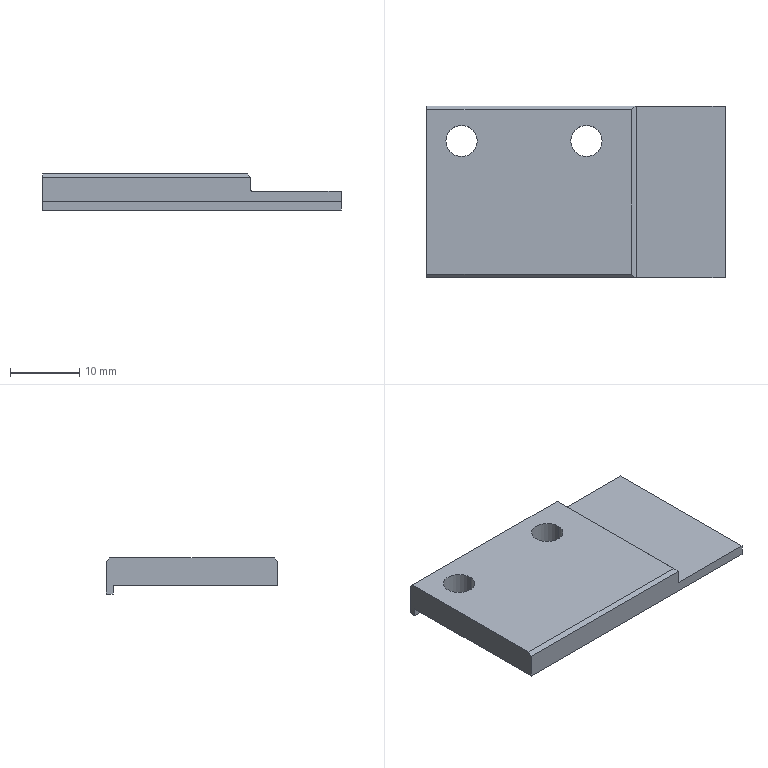Part | NX | 1 solid | 18 faces | box 43 x 24.7 x 5.2 mm | volume 3360 mm3 | plane 13 | cylinder 5 | commonest cylinder face diameters 4.5 x4 0.4 x1
STEP:
#1=CARTESIAN_POINT('',(0.,0.,-0.2));
#2=VERTEX_POINT('',#1);
#3=CARTESIAN_POINT('',(0.,-1.,-0.2));
#4=VERTEX_POINT('',#3);
#5=CARTESIAN_POINT('',(0.,0.,-0.2));
#6=DIRECTION('',(0.,-1.,0.));
#7=VECTOR('',#6,1000.);
#8=LINE('',#5,#7);
#9=EDGE_CURVE('',#2,#4,#8,.T.);
#10=ORIENTED_EDGE('',*,*,#9,.F.);
#11=CARTESIAN_POINT('',(43.,0.,-0.2));
#12=VERTEX_POINT('',#11);
#13=CARTESIAN_POINT('',(0.,0.,-0.2));
#14=DIRECTION('',(1.,0.,0.));
#15=VECTOR('',#14,1000.);
#16=LINE('',#13,#15);
#17=EDGE_CURVE('',#2,#12,#16,.T.);
#18=ORIENTED_EDGE('',*,*,#17,.T.);
#19=CARTESIAN_POINT('',(43.,-1.,-0.2));
#20=VERTEX_POINT('',#19);
#21=CARTESIAN_POINT('',(43.,0.,-0.2));
#22=DIRECTION('',(0.,-1.,0.));
#23=VECTOR('',#22,1000.);
#24=LINE('',#21,#23);
#25=EDGE_CURVE('',#12,#20,#24,.T.);
#26=ORIENTED_EDGE('',*,*,#25,.T.);
#27=CARTESIAN_POINT('',(0.,-1.,-0.2));
#28=DIRECTION('',(-1.,0.,0.));
#29=VECTOR('',#28,1000.);
#30=LINE('',#27,#29);
#31=EDGE_CURVE('',#20,#4,#30,.T.);
#32=ORIENTED_EDGE('',*,*,#31,.T.);
#33=EDGE_LOOP('',(#10,#18,#26,#32));
#34=FACE_BOUND('',#33,.T.);
#35=CARTESIAN_POINT('',(0.,0.,-0.2));
#36=DIRECTION('',(0.,0.,1.));
#37=DIRECTION('',(1.,0.,0.));
#38=AXIS2_PLACEMENT_3D('',#35,#36,#37);
#39=PLANE('',#38);
#40=ADVANCED_FACE('',(#34),#39,.F.);
#41=ORIENTED_EDGE('',*,*,#9,.T.);
#42=CARTESIAN_POINT('',(0.,-1.,1.));
#43=VERTEX_POINT('',#42);
#44=CARTESIAN_POINT('',(0.,-1.,0.));
#45=DIRECTION('',(0.,0.,-1.));
#46=VECTOR('',#45,1000.);
#47=LINE('',#44,#46);
#48=EDGE_CURVE('',#43,#4,#47,.T.);
#49=ORIENTED_EDGE('',*,*,#48,.F.);
#50=CARTESIAN_POINT('',(0.,-24.7,1.));
#51=VERTEX_POINT('',#50);
#52=CARTESIAN_POINT('',(0.,0.,1.));
#53=DIRECTION('',(0.,-1.,0.));
#54=VECTOR('',#53,1000.);
#55=LINE('',#52,#54);
#56=EDGE_CURVE('',#43,#51,#55,.T.);
#57=ORIENTED_EDGE('',*,*,#56,.T.);
#58=CARTESIAN_POINT('',(0.,-24.7,4.5));
#59=VERTEX_POINT('',#58);
#60=CARTESIAN_POINT('',(0.,-24.7,0.));
#61=DIRECTION('',(0.,0.,-1.));
#62=VECTOR('',#61,1000.);
#63=LINE('',#60,#62);
#64=EDGE_CURVE('',#59,#51,#63,.T.);
#65=ORIENTED_EDGE('',*,*,#64,.F.);
#66=CARTESIAN_POINT('',(0.,-24.2,5.));
#67=VERTEX_POINT('',#66);
#68=CARTESIAN_POINT('',(0.,-29.2,0.));
#69=DIRECTION('',(0.,0.7071,0.7071));
#70=VECTOR('',#69,1000.);
#71=LINE('',#68,#70);
#72=EDGE_CURVE('',#59,#67,#71,.T.);
#73=ORIENTED_EDGE('',*,*,#72,.T.);
#74=CARTESIAN_POINT('',(0.,-0.5,5.));
#75=VERTEX_POINT('',#74);
#76=CARTESIAN_POINT('',(0.,0.,5.));
#77=DIRECTION('',(0.,-1.,0.));
#78=VECTOR('',#77,1000.);
#79=LINE('',#76,#78);
#80=EDGE_CURVE('',#75,#67,#79,.T.);
#81=ORIENTED_EDGE('',*,*,#80,.F.);
#82=CARTESIAN_POINT('',(0.,0.,4.5));
#83=VERTEX_POINT('',#82);
#84=CARTESIAN_POINT('',(0.,4.5,0.));
#85=DIRECTION('',(0.,-0.7071,0.7071));
#86=VECTOR('',#85,1000.);
#87=LINE('',#84,#86);
#88=EDGE_CURVE('',#83,#75,#87,.T.);
#89=ORIENTED_EDGE('',*,*,#88,.F.);
#90=CARTESIAN_POINT('',(0.,0.,0.));
#91=DIRECTION('',(0.,0.,1.));
#92=VECTOR('',#91,1000.);
#93=LINE('',#90,#92);
#94=EDGE_CURVE('',#2,#83,#93,.T.);
#95=ORIENTED_EDGE('',*,*,#94,.F.);
#96=EDGE_LOOP('',(#41,#49,#57,#65,#73,#81,#89,#95));
#97=FACE_BOUND('',#96,.T.);
#98=CARTESIAN_POINT('',(0.,0.,0.));
#99=DIRECTION('',(-1.,0.,0.));
#100=DIRECTION('',(0.,0.,1.));
#101=AXIS2_PLACEMENT_3D('',#98,#99,#100);
#102=PLANE('',#101);
#103=ADVANCED_FACE('',(#97),#102,.T.);
#104=CARTESIAN_POINT('',(30.,0.,4.5));
#105=VERTEX_POINT('',#104);
#106=CARTESIAN_POINT('',(0.,0.,4.5));
#107=DIRECTION('',(-1.,0.,0.));
#108=VECTOR('',#107,1000.);
#109=LINE('',#106,#108);
#110=EDGE_CURVE('',#105,#83,#109,.T.);
#111=ORIENTED_EDGE('',*,*,#110,.F.);
#112=CARTESIAN_POINT('',(30.,0.,2.7));
#113=VERTEX_POINT('',#112);
#114=CARTESIAN_POINT('',(30.,0.,0.));
#115=DIRECTION('',(0.,0.,-1.));
#116=VECTOR('',#115,1000.);
#117=LINE('',#114,#116);
#118=EDGE_CURVE('',#105,#113,#117,.T.);
#119=ORIENTED_EDGE('',*,*,#118,.T.);
#120=CARTESIAN_POINT('',(30.2,0.,2.5));
#121=VERTEX_POINT('',#120);
#122=CARTESIAN_POINT('',(30.2,0.,2.7));
#123=DIRECTION('',(0.,1.,0.));
#124=DIRECTION('',(0.,0.,-1.));
#125=AXIS2_PLACEMENT_3D('',#122,#123,#124);
#126=CIRCLE('',#125,0.2);
#127=EDGE_CURVE('',#121,#113,#126,.T.);
#128=ORIENTED_EDGE('',*,*,#127,.F.);
#129=CARTESIAN_POINT('',(43.,0.,2.5));
#130=VERTEX_POINT('',#129);
#131=CARTESIAN_POINT('',(0.,0.,2.5));
#132=DIRECTION('',(-1.,0.,0.));
#133=VECTOR('',#132,1000.);
#134=LINE('',#131,#133);
#135=EDGE_CURVE('',#130,#121,#134,.T.);
#136=ORIENTED_EDGE('',*,*,#135,.F.);
#137=CARTESIAN_POINT('',(43.,0.,0.));
#138=DIRECTION('',(0.,0.,1.));
#139=VECTOR('',#138,1000.);
#140=LINE('',#137,#139);
#141=EDGE_CURVE('',#12,#130,#140,.T.);
#142=ORIENTED_EDGE('',*,*,#141,.F.);
#143=ORIENTED_EDGE('',*,*,#17,.F.);
#144=ORIENTED_EDGE('',*,*,#94,.T.);
#145=EDGE_LOOP('',(#111,#119,#128,#136,#142,#143,#144));
#146=FACE_BOUND('',#145,.T.);
#147=CARTESIAN_POINT('',(43.,0.,0.));
#148=DIRECTION('',(0.,1.,0.));
#149=DIRECTION('',(1.,0.,0.));
#150=AXIS2_PLACEMENT_3D('',#147,#148,#149);
#151=PLANE('',#150);
#152=ADVANCED_FACE('',(#146),#151,.T.);
#153=CARTESIAN_POINT('',(30.2,-24.7,2.5));
#154=VERTEX_POINT('',#153);
#155=CARTESIAN_POINT('',(30.2,-26.782,2.5));
#156=DIRECTION('',(0.,1.,0.));
#157=VECTOR('',#156,1000.);
#158=LINE('',#155,#157);
#159=EDGE_CURVE('',#154,#121,#158,.T.);
#160=ORIENTED_EDGE('',*,*,#159,.F.);
#161=CARTESIAN_POINT('',(43.,-24.7,2.5));
#162=VERTEX_POINT('',#161);
#163=CARTESIAN_POINT('',(0.,-24.7,2.5));
#164=DIRECTION('',(-1.,0.,0.));
#165=VECTOR('',#164,1000.);
#166=LINE('',#163,#165);
#167=EDGE_CURVE('',#162,#154,#166,.T.);
#168=ORIENTED_EDGE('',*,*,#167,.F.);
#169=CARTESIAN_POINT('',(43.,0.,2.5));
#170=DIRECTION('',(0.,1.,0.));
#171=VECTOR('',#170,1000.);
#172=LINE('',#169,#171);
#173=EDGE_CURVE('',#162,#130,#172,.T.);
#174=ORIENTED_EDGE('',*,*,#173,.T.);
#175=ORIENTED_EDGE('',*,*,#135,.T.);
#176=EDGE_LOOP('',(#160,#168,#174,#175));
#177=FACE_BOUND('',#176,.T.);
#178=CARTESIAN_POINT('',(0.,0.,2.5));
#179=DIRECTION('',(0.,0.,1.));
#180=DIRECTION('',(1.,0.,0.));
#181=AXIS2_PLACEMENT_3D('',#178,#179,#180);
#182=PLANE('',#181);
#183=ADVANCED_FACE('',(#177),#182,.T.);
#184=ORIENTED_EDGE('',*,*,#159,.T.);
#185=ORIENTED_EDGE('',*,*,#127,.T.);
#186=CARTESIAN_POINT('',(30.,-24.7,2.7));
#187=VERTEX_POINT('',#186);
#188=CARTESIAN_POINT('',(30.,-26.7,2.7));
#189=DIRECTION('',(0.,1.,0.));
#190=VECTOR('',#189,1000.);
#191=LINE('',#188,#190);
#192=EDGE_CURVE('',#187,#113,#191,.T.);
#193=ORIENTED_EDGE('',*,*,#192,.F.);
#194=CARTESIAN_POINT('',(30.2,-24.7,2.7));
#195=DIRECTION('',(0.,1.,0.));
#196=DIRECTION('',(0.,0.,-1.));
#197=AXIS2_PLACEMENT_3D('',#194,#195,#196);
#198=CIRCLE('',#197,0.2);
#199=EDGE_CURVE('',#154,#187,#198,.T.);
#200=ORIENTED_EDGE('',*,*,#199,.F.);
#201=EDGE_LOOP('',(#184,#185,#193,#200));
#202=FACE_BOUND('',#201,.T.);
#203=CARTESIAN_POINT('',(30.2,-26.782,2.7));
#204=DIRECTION('',(0.,1.,0.));
#205=DIRECTION('',(0.,0.,-1.));
#206=AXIS2_PLACEMENT_3D('',#203,#204,#205);
#207=CYLINDRICAL_SURFACE('',#206,0.2);
#208=ADVANCED_FACE('',(#202),#207,.F.);
#209=CARTESIAN_POINT('',(30.,-24.7,4.5));
#210=VERTEX_POINT('',#209);
#211=CARTESIAN_POINT('',(0.,-24.7,4.5));
#212=DIRECTION('',(-1.,0.,0.));
#213=VECTOR('',#212,1000.);
#214=LINE('',#211,#213);
#215=EDGE_CURVE('',#210,#59,#214,.T.);
#216=ORIENTED_EDGE('',*,*,#215,.T.);
#217=ORIENTED_EDGE('',*,*,#64,.T.);
#218=CARTESIAN_POINT('',(43.,-24.7,1.));
#219=VERTEX_POINT('',#218);
#220=CARTESIAN_POINT('',(0.,-24.7,1.));
#221=DIRECTION('',(-1.,0.,0.));
#222=VECTOR('',#221,1000.);
#223=LINE('',#220,#222);
#224=EDGE_CURVE('',#219,#51,#223,.T.);
#225=ORIENTED_EDGE('',*,*,#224,.F.);
#226=CARTESIAN_POINT('',(43.,-24.7,0.));
#227=DIRECTION('',(0.,0.,1.));
#228=VECTOR('',#227,1000.);
#229=LINE('',#226,#228);
#230=EDGE_CURVE('',#219,#162,#229,.T.);
#231=ORIENTED_EDGE('',*,*,#230,.T.);
#232=ORIENTED_EDGE('',*,*,#167,.T.);
#233=ORIENTED_EDGE('',*,*,#199,.T.);
#234=CARTESIAN_POINT('',(30.,-24.7,0.));
#235=DIRECTION('',(0.,0.,1.));
#236=VECTOR('',#235,1000.);
#237=LINE('',#234,#236);
#238=EDGE_CURVE('',#187,#210,#237,.T.);
#239=ORIENTED_EDGE('',*,*,#238,.T.);
#240=EDGE_LOOP('',(#216,#217,#225,#231,#232,#233,#239));
#241=FACE_BOUND('',#240,.T.);
#242=CARTESIAN_POINT('',(0.,-24.7,0.));
#243=DIRECTION('',(0.,-1.,0.));
#244=DIRECTION('',(0.,0.,-1.));
#245=AXIS2_PLACEMENT_3D('',#242,#243,#244);
#246=PLANE('',#245);
#247=ADVANCED_FACE('',(#241),#246,.T.);
#248=CARTESIAN_POINT('',(30.,0.,4.5));
#249=DIRECTION('',(0.,1.,0.));
#250=VECTOR('',#249,1000.);
#251=LINE('',#248,#250);
#252=EDGE_CURVE('',#210,#105,#251,.T.);
#253=ORIENTED_EDGE('',*,*,#252,.F.);
#254=ORIENTED_EDGE('',*,*,#238,.F.);
#255=ORIENTED_EDGE('',*,*,#192,.T.);
#256=ORIENTED_EDGE('',*,*,#118,.F.);
#257=EDGE_LOOP('',(#253,#254,#255,#256));
#258=FACE_BOUND('',#257,.T.);
#259=CARTESIAN_POINT('',(30.,0.,5.));
#260=DIRECTION('',(-1.,0.,0.));
#261=DIRECTION('',(0.,0.,1.));
#262=AXIS2_PLACEMENT_3D('',#259,#260,#261);
#263=PLANE('',#262);
#264=ADVANCED_FACE('',(#258),#263,.F.);
#265=CARTESIAN_POINT('',(29.5,-24.2,5.));
#266=VERTEX_POINT('',#265);
#267=CARTESIAN_POINT('',(29.5,-0.5,5.));
#268=VERTEX_POINT('',#267);
#269=CARTESIAN_POINT('',(29.5,0.,5.));
#270=DIRECTION('',(0.,1.,0.));
#271=VECTOR('',#270,1000.);
#272=LINE('',#269,#271);
#273=EDGE_CURVE('',#266,#268,#272,.T.);
#274=ORIENTED_EDGE('',*,*,#273,.T.);
#275=CARTESIAN_POINT('',(0.,-0.5,5.));
#276=DIRECTION('',(1.,0.,0.));
#277=VECTOR('',#276,1000.);
#278=LINE('',#275,#277);
#279=EDGE_CURVE('',#75,#268,#278,.T.);
#280=ORIENTED_EDGE('',*,*,#279,.F.);
#281=ORIENTED_EDGE('',*,*,#80,.T.);
#282=CARTESIAN_POINT('',(0.,-24.2,5.));
#283=DIRECTION('',(1.,0.,0.));
#284=VECTOR('',#283,1000.);
#285=LINE('',#282,#284);
#286=EDGE_CURVE('',#67,#266,#285,.T.);
#287=ORIENTED_EDGE('',*,*,#286,.T.);
#288=EDGE_LOOP('',(#274,#280,#281,#287));
#289=FACE_BOUND('',#288,.T.);
#290=CARTESIAN_POINT('',(20.75,-5.,5.));
#291=VERTEX_POINT('',#290);
#292=CARTESIAN_POINT('',(25.25,-5.,5.));
#293=VERTEX_POINT('',#292);
#294=CARTESIAN_POINT('',(23.,-5.,5.));
#295=DIRECTION('',(0.,0.,-1.));
#296=DIRECTION('',(-1.,0.,0.));
#297=AXIS2_PLACEMENT_3D('',#294,#295,#296);
#298=CIRCLE('',#297,2.25);
#299=EDGE_CURVE('',#291,#293,#298,.T.);
#300=ORIENTED_EDGE('',*,*,#299,.T.);
#301=CARTESIAN_POINT('',(23.,-5.,5.));
#302=DIRECTION('',(0.,0.,-1.));
#303=DIRECTION('',(-1.,0.,0.));
#304=AXIS2_PLACEMENT_3D('',#301,#302,#303);
#305=CIRCLE('',#304,2.25);
#306=EDGE_CURVE('',#293,#291,#305,.T.);
#307=ORIENTED_EDGE('',*,*,#306,.T.);
#308=EDGE_LOOP('',(#300,#307));
#309=FACE_BOUND('',#308,.T.);
#310=CARTESIAN_POINT('',(7.25,-5.,5.));
#311=VERTEX_POINT('',#310);
#312=CARTESIAN_POINT('',(2.75,-5.,5.));
#313=VERTEX_POINT('',#312);
#314=CARTESIAN_POINT('',(5.,-5.,5.));
#315=DIRECTION('',(0.,0.,-1.));
#316=DIRECTION('',(-1.,0.,0.));
#317=AXIS2_PLACEMENT_3D('',#314,#315,#316);
#318=CIRCLE('',#317,2.25);
#319=EDGE_CURVE('',#311,#313,#318,.T.);
#320=ORIENTED_EDGE('',*,*,#319,.T.);
#321=CARTESIAN_POINT('',(5.,-5.,5.));
#322=DIRECTION('',(0.,0.,-1.));
#323=DIRECTION('',(-1.,0.,0.));
#324=AXIS2_PLACEMENT_3D('',#321,#322,#323);
#325=CIRCLE('',#324,2.25);
#326=EDGE_CURVE('',#313,#311,#325,.T.);
#327=ORIENTED_EDGE('',*,*,#326,.T.);
#328=EDGE_LOOP('',(#320,#327));
#329=FACE_BOUND('',#328,.T.);
#330=CARTESIAN_POINT('',(0.,0.,5.));
#331=DIRECTION('',(0.,0.,1.));
#332=DIRECTION('',(1.,0.,0.));
#333=AXIS2_PLACEMENT_3D('',#330,#331,#332);
#334=PLANE('',#333);
#335=ADVANCED_FACE('',(#289,#309,#329),#334,.T.);
#336=CARTESIAN_POINT('',(25.25,-5.,1.));
#337=VERTEX_POINT('',#336);
#338=CARTESIAN_POINT('',(20.75,-5.,1.));
#339=VERTEX_POINT('',#338);
#340=CARTESIAN_POINT('',(23.,-5.,1.));
#341=DIRECTION('',(0.,0.,-1.));
#342=DIRECTION('',(-1.,0.,0.));
#343=AXIS2_PLACEMENT_3D('',#340,#341,#342);
#344=CIRCLE('',#343,2.25);
#345=EDGE_CURVE('',#337,#339,#344,.T.);
#346=ORIENTED_EDGE('',*,*,#345,.T.);
#347=CARTESIAN_POINT('',(20.75,-5.,5.));
#348=DIRECTION('',(0.,0.,-1.));
#349=VECTOR('',#348,1000.);
#350=LINE('',#347,#349);
#351=EDGE_CURVE('',#339,#291,#350,.F.);
#352=ORIENTED_EDGE('',*,*,#351,.T.);
#353=ORIENTED_EDGE('',*,*,#306,.F.);
#354=CARTESIAN_POINT('',(25.25,-5.,5.));
#355=DIRECTION('',(0.,0.,-1.));
#356=VECTOR('',#355,1000.);
#357=LINE('',#354,#356);
#358=EDGE_CURVE('',#337,#293,#357,.F.);
#359=ORIENTED_EDGE('',*,*,#358,.F.);
#360=EDGE_LOOP('',(#346,#352,#353,#359));
#361=FACE_BOUND('',#360,.T.);
#362=CARTESIAN_POINT('',(23.,-5.,5.));
#363=DIRECTION('',(0.,0.,-1.));
#364=DIRECTION('',(-1.,0.,0.));
#365=AXIS2_PLACEMENT_3D('',#362,#363,#364);
#366=CYLINDRICAL_SURFACE('',#365,2.25);
#367=ADVANCED_FACE('',(#361),#366,.F.);
#368=ORIENTED_EDGE('',*,*,#319,.F.);
#369=CARTESIAN_POINT('',(7.25,-5.,1.));
#370=VERTEX_POINT('',#369);
#371=CARTESIAN_POINT('',(7.25,-5.,5.));
#372=DIRECTION('',(0.,0.,-1.));
#373=VECTOR('',#372,1000.);
#374=LINE('',#371,#373);
#375=EDGE_CURVE('',#311,#370,#374,.T.);
#376=ORIENTED_EDGE('',*,*,#375,.T.);
#377=CARTESIAN_POINT('',(2.75,-5.,1.));
#378=VERTEX_POINT('',#377);
#379=CARTESIAN_POINT('',(5.,-5.,1.));
#380=DIRECTION('',(0.,0.,-1.));
#381=DIRECTION('',(-1.,0.,0.));
#382=AXIS2_PLACEMENT_3D('',#379,#380,#381);
#383=CIRCLE('',#382,2.25);
#384=EDGE_CURVE('',#370,#378,#383,.T.);
#385=ORIENTED_EDGE('',*,*,#384,.T.);
#386=CARTESIAN_POINT('',(2.75,-5.,5.));
#387=DIRECTION('',(0.,0.,-1.));
#388=VECTOR('',#387,1000.);
#389=LINE('',#386,#388);
#390=EDGE_CURVE('',#313,#378,#389,.T.);
#391=ORIENTED_EDGE('',*,*,#390,.F.);
#392=EDGE_LOOP('',(#368,#376,#385,#391));
#393=FACE_BOUND('',#392,.T.);
#394=CARTESIAN_POINT('',(5.,-5.,5.));
#395=DIRECTION('',(0.,0.,-1.));
#396=DIRECTION('',(-1.,0.,0.));
#397=AXIS2_PLACEMENT_3D('',#394,#395,#396);
#398=CYLINDRICAL_SURFACE('',#397,2.25);
#399=ADVANCED_FACE('',(#393),#398,.F.);
#400=ORIENTED_EDGE('',*,*,#56,.F.);
#401=CARTESIAN_POINT('',(43.,-1.,1.));
#402=VERTEX_POINT('',#401);
#403=CARTESIAN_POINT('',(0.,-1.,1.));
#404=DIRECTION('',(-1.,0.,0.));
#405=VECTOR('',#404,1000.);
#406=LINE('',#403,#405);
#407=EDGE_CURVE('',#402,#43,#406,.T.);
#408=ORIENTED_EDGE('',*,*,#407,.F.);
#409=CARTESIAN_POINT('',(43.,0.,1.));
#410=DIRECTION('',(0.,1.,0.));
#411=VECTOR('',#410,1000.);
#412=LINE('',#409,#411);
#413=EDGE_CURVE('',#219,#402,#412,.T.);
#414=ORIENTED_EDGE('',*,*,#413,.F.);
#415=ORIENTED_EDGE('',*,*,#224,.T.);
#416=EDGE_LOOP('',(#400,#408,#414,#415));
#417=FACE_BOUND('',#416,.T.);
#418=ORIENTED_EDGE('',*,*,#345,.F.);
#419=CARTESIAN_POINT('',(23.,-5.,1.));
#420=DIRECTION('',(0.,0.,-1.));
#421=DIRECTION('',(-1.,0.,0.));
#422=AXIS2_PLACEMENT_3D('',#419,#420,#421);
#423=CIRCLE('',#422,2.25);
#424=EDGE_CURVE('',#339,#337,#423,.T.);
#425=ORIENTED_EDGE('',*,*,#424,.F.);
#426=EDGE_LOOP('',(#418,#425));
#427=FACE_BOUND('',#426,.T.);
#428=CARTESIAN_POINT('',(5.,-5.,1.));
#429=DIRECTION('',(0.,0.,-1.));
#430=DIRECTION('',(-1.,0.,0.));
#431=AXIS2_PLACEMENT_3D('',#428,#429,#430);
#432=CIRCLE('',#431,2.25);
#433=EDGE_CURVE('',#378,#370,#432,.T.);
#434=ORIENTED_EDGE('',*,*,#433,.F.);
#435=ORIENTED_EDGE('',*,*,#384,.F.);
#436=EDGE_LOOP('',(#434,#435));
#437=FACE_BOUND('',#436,.T.);
#438=CARTESIAN_POINT('',(0.,-26.7,1.));
#439=DIRECTION('',(0.,0.,1.));
#440=DIRECTION('',(1.,0.,0.));
#441=AXIS2_PLACEMENT_3D('',#438,#439,#440);
#442=PLANE('',#441);
#443=ADVANCED_FACE('',(#417,#427,#437),#442,.F.);
#444=ORIENTED_EDGE('',*,*,#173,.F.);
#445=ORIENTED_EDGE('',*,*,#230,.F.);
#446=ORIENTED_EDGE('',*,*,#413,.T.);
#447=CARTESIAN_POINT('',(43.,-1.,0.));
#448=DIRECTION('',(0.,0.,1.));
#449=VECTOR('',#448,1000.);
#450=LINE('',#447,#449);
#451=EDGE_CURVE('',#20,#402,#450,.T.);
#452=ORIENTED_EDGE('',*,*,#451,.F.);
#453=ORIENTED_EDGE('',*,*,#25,.F.);
#454=ORIENTED_EDGE('',*,*,#141,.T.);
#455=EDGE_LOOP('',(#444,#445,#446,#452,#453,#454));
#456=FACE_BOUND('',#455,.T.);
#457=CARTESIAN_POINT('',(43.,-26.7,0.));
#458=DIRECTION('',(1.,0.,0.));
#459=DIRECTION('',(0.,1.,0.));
#460=AXIS2_PLACEMENT_3D('',#457,#458,#459);
#461=PLANE('',#460);
#462=ADVANCED_FACE('',(#456),#461,.T.);
#463=ORIENTED_EDGE('',*,*,#31,.F.);
#464=ORIENTED_EDGE('',*,*,#451,.T.);
#465=ORIENTED_EDGE('',*,*,#407,.T.);
#466=ORIENTED_EDGE('',*,*,#48,.T.);
#467=EDGE_LOOP('',(#463,#464,#465,#466));
#468=FACE_BOUND('',#467,.T.);
#469=CARTESIAN_POINT('',(0.,-1.,1.));
#470=DIRECTION('',(0.,1.,0.));
#471=DIRECTION('',(1.,0.,0.));
#472=AXIS2_PLACEMENT_3D('',#469,#470,#471);
#473=PLANE('',#472);
#474=ADVANCED_FACE('',(#468),#473,.F.);
#475=ORIENTED_EDGE('',*,*,#110,.T.);
#476=ORIENTED_EDGE('',*,*,#88,.T.);
#477=ORIENTED_EDGE('',*,*,#279,.T.);
#478=CARTESIAN_POINT('',(34.5,4.5,0.));
#479=DIRECTION('',(0.5774,0.5774,-0.5774));
#480=VECTOR('',#479,1000.);
#481=LINE('',#478,#480);
#482=EDGE_CURVE('',#268,#105,#481,.T.);
#483=ORIENTED_EDGE('',*,*,#482,.T.);
#484=EDGE_LOOP('',(#475,#476,#477,#483));
#485=FACE_BOUND('',#484,.T.);
#486=CARTESIAN_POINT('',(15.,-0.25,4.75));
#487=DIRECTION('',(0.,0.7071,0.7071));
#488=DIRECTION('',(1.,0.,0.));
#489=AXIS2_PLACEMENT_3D('',#486,#487,#488);
#490=PLANE('',#489);
#491=ADVANCED_FACE('',(#485),#490,.T.);
#492=ORIENTED_EDGE('',*,*,#215,.F.);
#493=CARTESIAN_POINT('',(34.5,-29.2,0.));
#494=DIRECTION('',(0.5774,-0.5774,-0.5774));
#495=VECTOR('',#494,1000.);
#496=LINE('',#493,#495);
#497=EDGE_CURVE('',#266,#210,#496,.T.);
#498=ORIENTED_EDGE('',*,*,#497,.F.);
#499=ORIENTED_EDGE('',*,*,#286,.F.);
#500=ORIENTED_EDGE('',*,*,#72,.F.);
#501=EDGE_LOOP('',(#492,#498,#499,#500));
#502=FACE_BOUND('',#501,.T.);
#503=CARTESIAN_POINT('',(15.,-24.45,4.75));
#504=DIRECTION('',(0.,0.7071,-0.7071));
#505=DIRECTION('',(-1.,0.,0.));
#506=AXIS2_PLACEMENT_3D('',#503,#504,#505);
#507=PLANE('',#506);
#508=ADVANCED_FACE('',(#502),#507,.F.);
#509=ORIENTED_EDGE('',*,*,#252,.T.);
#510=ORIENTED_EDGE('',*,*,#482,.F.);
#511=ORIENTED_EDGE('',*,*,#273,.F.);
#512=ORIENTED_EDGE('',*,*,#497,.T.);
#513=EDGE_LOOP('',(#509,#510,#511,#512));
#514=FACE_BOUND('',#513,.T.);
#515=CARTESIAN_POINT('',(29.75,-12.35,4.75));
#516=DIRECTION('',(-0.7071,0.,-0.7071));
#517=DIRECTION('',(-0.7071,0.,0.7071));
#518=AXIS2_PLACEMENT_3D('',#515,#516,#517);
#519=PLANE('',#518);
#520=ADVANCED_FACE('',(#514),#519,.F.);
#521=ORIENTED_EDGE('',*,*,#433,.T.);
#522=ORIENTED_EDGE('',*,*,#375,.F.);
#523=ORIENTED_EDGE('',*,*,#326,.F.);
#524=ORIENTED_EDGE('',*,*,#390,.T.);
#525=EDGE_LOOP('',(#521,#522,#523,#524));
#526=FACE_BOUND('',#525,.T.);
#527=CARTESIAN_POINT('',(5.,-5.,5.));
#528=DIRECTION('',(0.,0.,-1.));
#529=DIRECTION('',(-1.,0.,0.));
#530=AXIS2_PLACEMENT_3D('',#527,#528,#529);
#531=CYLINDRICAL_SURFACE('',#530,2.25);
#532=ADVANCED_FACE('',(#526),#531,.F.);
#533=ORIENTED_EDGE('',*,*,#299,.F.);
#534=ORIENTED_EDGE('',*,*,#351,.F.);
#535=ORIENTED_EDGE('',*,*,#424,.T.);
#536=ORIENTED_EDGE('',*,*,#358,.T.);
#537=EDGE_LOOP('',(#533,#534,#535,#536));
#538=FACE_BOUND('',#537,.T.);
#539=CARTESIAN_POINT('',(23.,-5.,5.));
#540=DIRECTION('',(0.,0.,-1.));
#541=DIRECTION('',(-1.,0.,0.));
#542=AXIS2_PLACEMENT_3D('',#539,#540,#541);
#543=CYLINDRICAL_SURFACE('',#542,2.25);
#544=ADVANCED_FACE('',(#538),#543,.F.);
#545=CLOSED_SHELL('',(#40,#103,#152,#183,#208,#247,#264,#335,#367,#399,#443,#462,#474,#491,#508,#520,#532,#544));
#546=MANIFOLD_SOLID_BREP('',#545);
#547=(LENGTH_UNIT()NAMED_UNIT(*)SI_UNIT(.MILLI.,.METRE.));
#548=UNCERTAINTY_MEASURE_WITH_UNIT(LENGTH_MEASURE(0.00001),#547,'','');
#549=(NAMED_UNIT(*)PLANE_ANGLE_UNIT()SI_UNIT($,.RADIAN.));
#550=(NAMED_UNIT(*)SI_UNIT($,.STERADIAN.)SOLID_ANGLE_UNIT());
#551=(GEOMETRIC_REPRESENTATION_CONTEXT(3)GLOBAL_UNCERTAINTY_ASSIGNED_CONTEXT((#548))GLOBAL_UNIT_ASSIGNED_CONTEXT((#547,#549,#550))REPRESENTATION_CONTEXT('',''));
#552=ADVANCED_BREP_SHAPE_REPRESENTATION('',(#546),#551);